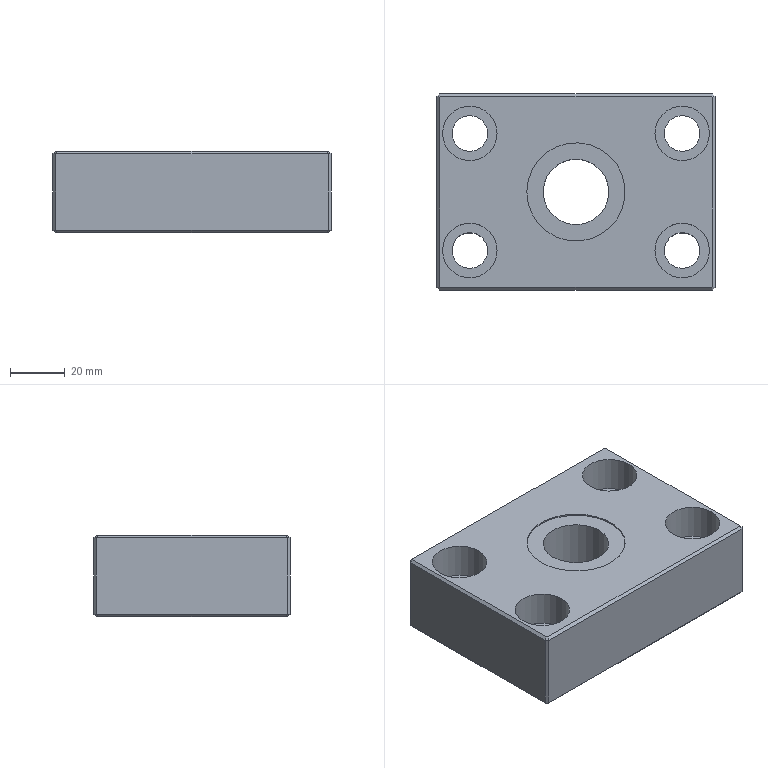NC program | NX | posted with a generic post | part box 102 x 72 x 30 mm
Whole program:
N10 G17 G21 G94 G90
(PLANAR_MILL_COPY_1 , TOOL : D80-FACE-MILL)
N12 T01 M6
N14 G54
N16 G17 G0 G90 X96. Y-0.5 S3500 M3
N18 G43 Z35. H1
N20 Z6.
N22 G94 G1 Z4. F1200.
N24 X53.
N26 X-53.
N28 X-96.
N30 Z6.
N32 G0 Z35.
N34 X96.
N36 Z5.
N38 G1 Z3.
N40 X53.
N42 X-53.
N44 X-96.
N46 Z5.
N48 G0 Z35.
N50 X96.
N52 Z4.
N54 G1 Z2.
N56 X53.
N58 X-53.
N60 X-96.
N62 Z4.
N64 G0 Z35.
N66 X96.
N68 Z3.
N70 G1 Z1.
N72 X53.
N74 X-53.
N76 X-96.
N78 Z3.
N80 G0 Z35.
N82 X96.
N84 Z2.03
N86 G1 Z0.03
N88 X53.
N90 X-53.
N92 X-96.
N94 Z2.03
N96 G0 Z35.
N98 M5
(PLANAR_MILL_5 , TOOL : D3-9-D4-50-3T-ROUGH)
N100 T09 M6
N102 G54
N104 G17 G0 G90 X-10.959 Y-26.704 S4500 M3
N106 G43 Z30. H9
N108 Z1.
N110 G94 G1 X-11.204 Y-26.618 Z0.999 F800.
N112 X-14.44 Y-25.011 Z0.99
N114 X-17.45 Y-23.012 Z0.98
N116 X-20.187 Y-20.653 Z0.971
N118 X-22.608 Y-17.97 Z0.961
N120 X-24.675 Y-15.006 Z0.952
N122 X-26.356 Y-11.807 Z0.943
N124 X-27.624 Y-8.424 Z0.933
N126 X-28.46 Y-4.908 Z0.924
N128 X-28.85 Y-1.316 Z0.914
N130 Y1.316 Z0.907
N132 X-28.46 Y4.908 Z0.898
N134 X-27.624 Y8.424 Z0.888
N136 X-26.356 Y11.807 Z0.879
N138 X-24.675 Y15.006 Z0.869
N140 X-22.608 Y17.97 Z0.86
N142 X-20.187 Y20.653 Z0.851
N144 X-17.45 Y23.012 Z0.841
N146 X-14.44 Y25.011 Z0.832
N148 X-11.204 Y26.618 Z0.822
N150 X-7.792 Y27.809 Z0.813
N152 X-4.258 Y28.564 Z0.803
N154 X-0.658 Y28.872 Z0.794
N156 X2.952 Y28.729 Z0.784
N158 X6.517 Y28.135 Z0.775
N160 X9.979 Y27.101 Z0.765
N162 X13.285 Y25.643 Z0.756
N164 X15.565 Y24.327 Z0.749
N166 X18.354 Y22.298 Z0.74
N168 X20.881 Y19.951 Z0.731
N170 X23.111 Y17.319 Z0.722
N172 X25.011 Y14.44 Z0.713
N174 X26.554 Y11.355 Z0.704
N176 X27.718 Y8.109 Z0.695
N178 X28.487 Y4.746 Z0.686
N180 X28.85 Y1.316 Z0.677
N182 Y-1.316 Z0.67
N184 X28.487 Y-4.746 Z0.661
N186 X27.718 Y-8.109 Z0.652
N188 X26.554 Y-11.355 Z0.643
N190 X25.011 Y-14.44 Z0.634
N192 X23.111 Y-17.319 Z0.625
N194 X20.881 Y-19.951 Z0.616
N196 X18.354 Y-22.298 Z0.607
N198 X15.565 Y-24.327 Z0.598
N200 X13.285 Y-25.643 Z0.591
N202 X9.979 Y-27.101 Z0.581
N204 X6.517 Y-28.135 Z0.572
N206 X2.952 Y-28.729 Z0.562
N208 X-0.658 Y-28.872 Z0.553
N210 X-4.258 Y-28.564 Z0.543
N212 X-7.792 Y-27.809 Z0.534
N214 X-11.204 Y-26.618 Z0.525
N216 X-14.44 Y-25.011 Z0.515
N218 X-17.45 Y-23.012 Z0.506
N220 X-20.187 Y-20.653 Z0.496
N222 X-22.608 Y-17.97 Z0.487
N224 X-24.675 Y-15.006 Z0.477
N226 X-26.356 Y-11.807 Z0.468
N228 X-27.624 Y-8.424 Z0.458
N230 X-28.46 Y-4.908 Z0.449
N232 X-28.85 Y-1.316 Z0.439
N234 Y1.316 Z0.433
N236 X-28.46 Y4.908 Z0.423
N238 X-27.624 Y8.424 Z0.414
N240 X-26.356 Y11.807 Z0.404
N242 X-24.675 Y15.006 Z0.395
N244 X-22.608 Y17.97 Z0.385
N246 X-20.187 Y20.653 Z0.376
N248 X-17.45 Y23.012 Z0.366
N250 X-14.44 Y25.011 Z0.357
N252 X-11.204 Y26.618 Z0.347
N254 X-7.792 Y27.809 Z0.338
N256 X-4.258 Y28.564 Z0.328
N258 X-0.658 Y28.872 Z0.319
N260 X2.952 Y28.729 Z0.31
N262 X6.517 Y28.135 Z0.3
N264 X9.979 Y27.101 Z0.291
N266 X13.285 Y25.643 Z0.281
N268 X15.565 Y24.327 Z0.274
N270 X18.354 Y22.298 Z0.265
N272 X20.881 Y19.951 Z0.256
N274 X23.111 Y17.319 Z0.247
N276 X25.011 Y14.44 Z0.238
N278 X26.554 Y11.355 Z0.229
N280 X27.718 Y8.109 Z0.22
N282 X28.487 Y4.746 Z0.211
N284 X28.85 Y1.316 Z0.202
N286 Y-1.316 Z0.195
N288 X28.487 Y-4.746 Z0.186
N290 X27.718 Y-8.109 Z0.177
N292 X26.554 Y-11.355 Z0.168
N294 X25.011 Y-14.44 Z0.159
N296 X23.111 Y-17.319 Z0.15
N298 X20.881 Y-19.951 Z0.141
N300 X18.354 Y-22.298 Z0.132
N302 X15.565 Y-24.327 Z0.123
N304 X13.285 Y-25.643 Z0.116
N306 X9.979 Y-27.101 Z0.107
N308 X6.517 Y-28.135 Z0.097
N310 X2.952 Y-28.729 Z0.088
N312 X-0.658 Y-28.872 Z0.078
N314 X-4.258 Y-28.564 Z0.069
N316 X-7.792 Y-27.809 Z0.059
N318 X-11.204 Y-26.618 Z0.05
N320 X-14.44 Y-25.011 Z0.04
N322 X-17.45 Y-23.012 Z0.031
N324 X-20.187 Y-20.653 Z0.021
N326 X-22.608 Y-17.97 Z0.012
N328 X-24.675 Y-15.006 Z0.002
N330 X-26.356 Y-11.807 Z-0.007
N332 X-27.624 Y-8.424 Z-0.016
N334 X-28.46 Y-4.908 Z-0.026
N336 X-28.85 Y-1.316 Z-0.035
N338 Y1.316 Z-0.042
N340 X-28.46 Y4.908 Z-0.052
N342 X-27.624 Y8.424 Z-0.061
N344 X-26.356 Y11.807 Z-0.071
N346 X-24.675 Y15.006 Z-0.08
N348 X-22.608 Y17.97 Z-0.09
N350 X-20.187 Y20.653 Z-0.099
N352 X-17.45 Y23.012 Z-0.108
N354 X-14.44 Y25.011 Z-0.118
N356 X-11.204 Y26.618 Z-0.127
N358 X-7.792 Y27.809 Z-0.137
N360 X-4.258 Y28.564 Z-0.146
N362 X-0.658 Y28.872 Z-0.156
N364 X2.952 Y28.729 Z-0.165
N366 X6.517 Y28.135 Z-0.175
N368 X9.979 Y27.101 Z-0.184
N370 X13.285 Y25.643 Z-0.194
N372 X15.565 Y24.327 Z-0.2
N374 X18.354 Y22.298 Z-0.21
N376 X20.881 Y19.951 Z-0.219
N378 X23.111 Y17.319 Z-0.228
N380 X25.011 Y14.44 Z-0.237
N382 X26.554 Y11.355 Z-0.246
N384 X27.718 Y8.109 Z-0.255
N386 X28.487 Y4.746 Z-0.264
N388 X28.85 Y1.316 Z-0.273
N390 Y-1.316 Z-0.28
N392 X28.487 Y-4.746 Z-0.289
N394 X27.718 Y-8.109 Z-0.298
N396 X26.554 Y-11.355 Z-0.307
N398 X25.011 Y-14.44 Z-0.316
N400 X23.111 Y-17.319 Z-0.325
N402 X20.881 Y-19.951 Z-0.334
N404 X18.354 Y-22.298 Z-0.343
N406 X15.565 Y-24.327 Z-0.352
N408 X13.285 Y-25.643 Z-0.359
N410 X9.979 Y-27.101 Z-0.368
N412 X6.517 Y-28.135 Z-0.378
N414 X2.952 Y-28.729 Z-0.387
N416 X-0.658 Y-28.872 Z-0.397
N418 X-4.258 Y-28.564 Z-0.406
N420 X-7.792 Y-27.809 Z-0.416
N422 X-11.204 Y-26.618 Z-0.425
N424 X-14.44 Y-25.011 Z-0.434
N426 X-17.45 Y-23.012 Z-0.444
N428 X-20.187 Y-20.653 Z-0.453
N430 X-22.608 Y-17.97 Z-0.463
N432 X-24.675 Y-15.006 Z-0.472
N434 X-26.356 Y-11.807 Z-0.482
N436 X-27.624 Y-8.424 Z-0.491
N438 X-28.46 Y-4.908 Z-0.501
N440 X-28.85 Y-1.316 Z-0.51
N442 Y1.316 Z-0.517
N444 X-28.46 Y4.908 Z-0.526
N446 X-27.624 Y8.424 Z-0.536
N448 X-26.356 Y11.807 Z-0.545
N450 X-24.675 Y15.006 Z-0.555
N452 X-22.608 Y17.97 Z-0.564
N454 X-20.187 Y20.653 Z-0.574
N456 X-17.45 Y23.012 Z-0.583
N458 X-14.44 Y25.011 Z-0.593
N460 X-11.204 Y26.618 Z-0.602
N462 X-7.792 Y27.809 Z-0.612
N464 X-4.258 Y28.564 Z-0.621
N466 X-0.658 Y28.872 Z-0.631
N468 X2.952 Y28.729 Z-0.64
N470 X6.517 Y28.135 Z-0.649
N472 X9.979 Y27.101 Z-0.659
N474 X13.285 Y25.643 Z-0.668
N476 X15.565 Y24.327 Z-0.675
N478 X18.354 Y22.298 Z-0.684
N480 X20.881 Y19.951 Z-0.693
N482 X23.111 Y17.319 Z-0.702
N484 X25.011 Y14.44 Z-0.711
N486 X26.554 Y11.355 Z-0.72
N488 X27.718 Y8.109 Z-0.729
N490 X28.487 Y4.746 Z-0.738
N492 X28.85 Y1.316 Z-0.747
N494 Y-1.316 Z-0.754
N496 X28.487 Y-4.746 Z-0.763
N498 X27.718 Y-8.109 Z-0.772
N500 X26.554 Y-11.355 Z-0.781
N502 X25.011 Y-14.44 Z-0.791
N504 X23.111 Y-17.319 Z-0.8
N506 X20.881 Y-19.951 Z-0.809
N508 X18.354 Y-22.298 Z-0.818
N510 X15.565 Y-24.327 Z-0.827
N512 X13.285 Y-25.643 Z-0.834
N514 X9.979 Y-27.101 Z-0.843
N516 X6.517 Y-28.135 Z-0.852
N518 X2.952 Y-28.729 Z-0.862
N520 X-0.658 Y-28.872 Z-0.871
N522 X-4.258 Y-28.564 Z-0.881
N524 X-7.792 Y-27.809 Z-0.89
N526 X-11.204 Y-26.618 Z-0.9
N528 X-14.44 Y-25.011 Z-0.909
N530 X-17.45 Y-23.012 Z-0.919
N532 X-20.187 Y-20.653 Z-0.928
N534 X-22.608 Y-17.97 Z-0.938
N536 X-24.675 Y-15.006 Z-0.947
N538 X-26.356 Y-11.807 Z-0.956
N540 X-27.624 Y-8.424 Z-0.966
N542 X-28.46 Y-4.908 Z-0.975
N544 X-28.85 Y-1.316 Z-0.985
N546 Y1.316 Z-0.992
N548 X-28.46 Y4.908 Z-1.001
N550 X-27.624 Y8.424 Z-1.011
N552 X-26.356 Y11.807 Z-1.02
N554 X-24.675 Y15.006 Z-1.03
N556 X-22.608 Y17.97 Z-1.039
N558 X-20.187 Y20.653 Z-1.049
N560 X-17.45 Y23.012 Z-1.058
N562 X-14.44 Y25.011 Z-1.067
N564 X-11.204 Y26.618 Z-1.077
N566 X-7.792 Y27.809 Z-1.086
N568 X-4.258 Y28.564 Z-1.096
N570 X-0.658 Y28.872 Z-1.105
N572 X2.952 Y28.729 Z-1.115
N574 X6.517 Y28.135 Z-1.124
N576 X9.979 Y27.101 Z-1.134
N578 X13.285 Y25.643 Z-1.143
N580 X15.565 Y24.327 Z-1.15
N582 X18.354 Y22.298 Z-1.159
N584 X20.881 Y19.951 Z-1.168
N586 X23.111 Y17.319 Z-1.177
N588 X25.011 Y14.44 Z-1.186
N590 X26.554 Y11.355 Z-1.195
N592 X27.718 Y8.109 Z-1.204
N594 X28.487 Y4.746 Z-1.213
N596 X28.85 Y1.316 Z-1.222
N598 Y-1.316 Z-1.229
N600 X28.487 Y-4.746 Z-1.238
N602 X27.718 Y-8.109 Z-1.247
N604 X26.554 Y-11.355 Z-1.256
N606 X25.011 Y-14.44 Z-1.265
N608 X23.111 Y-17.319 Z-1.274
N610 X20.881 Y-19.951 Z-1.283
N612 X18.354 Y-22.298 Z-1.292
N614 X15.565 Y-24.327 Z-1.301
N616 X13.285 Y-25.643 Z-1.308
N618 X9.979 Y-27.101 Z-1.318
N620 X6.517 Y-28.135 Z-1.327
N622 X2.952 Y-28.729 Z-1.337
N624 X-0.658 Y-28.872 Z-1.346
N626 X-4.258 Y-28.564 Z-1.356
N628 X-7.792 Y-27.809 Z-1.365
N630 X-11.204 Y-26.618 Z-1.375
N632 X-14.44 Y-25.011 Z-1.384
N634 X-17.45 Y-23.012 Z-1.393
N636 X-20.187 Y-20.653 Z-1.403
N638 X-22.608 Y-17.97 Z-1.412
N640 X-24.675 Y-15.006 Z-1.422
N642 X-26.356 Y-11.807 Z-1.431
N644 X-27.624 Y-8.424 Z-1.441
N646 X-28.46 Y-4.908 Z-1.45
N648 X-28.85 Y-1.316 Z-1.46
N650 Y1.316 Z-1.467
N652 X-28.46 Y4.908 Z-1.476
N654 X-27.624 Y8.424 Z-1.485
N656 X-26.356 Y11.807 Z-1.495
N658 X-24.675 Y15.006 Z-1.504
N660 X-22.608 Y17.97 Z-1.514
N662 X-20.187 Y20.653 Z-1.523
N664 X-17.45 Y23.012 Z-1.533
N666 X-14.44 Y25.011 Z-1.542
N668 X-11.204 Y26.618 Z-1.552
N670 X-7.792 Y27.809 Z-1.561
N672 X-4.258 Y28.564 Z-1.571
N674 X-0.658 Y28.872 Z-1.58
N676 X2.952 Y28.729 Z-1.59
N678 X6.517 Y28.135 Z-1.599
N680 X9.979 Y27.101 Z-1.608
N682 X13.285 Y25.643 Z-1.618
N684 X15.565 Y24.327 Z-1.625
N686 X18.354 Y22.298 Z-1.634
N688 X20.881 Y19.951 Z-1.643
N690 X23.111 Y17.319 Z-1.652
N692 X25.011 Y14.44 Z-1.661
N694 X26.554 Y11.355 Z-1.67
N696 X27.718 Y8.109 Z-1.679
N698 X28.487 Y4.746 Z-1.688
N700 X28.85 Y1.316 Z-1.697
N702 Y-1.316 Z-1.704
N704 X28.487 Y-4.746 Z-1.713
N706 X27.718 Y-8.109 Z-1.722
N708 X26.554 Y-11.355 Z-1.731
N710 X25.011 Y-14.44 Z-1.74
N712 X23.111 Y-17.319 Z-1.749
N714 X20.881 Y-19.951 Z-1.758
N716 X18.354 Y-22.298 Z-1.767
N718 X15.565 Y-24.327 Z-1.776
N720 X13.285 Y-25.643 Z-1.783
N722 X9.979 Y-27.101 Z-1.793
N724 X6.517 Y-28.135 Z-1.802
N726 X2.952 Y-28.729 Z-1.811
N728 X-0.658 Y-28.872 Z-1.821
N730 X-4.258 Y-28.564 Z-1.83
N732 X-7.792 Y-27.809 Z-1.84
N734 X-11.204 Y-26.618 Z-1.849
N736 X-14.44 Y-25.011 Z-1.859
N738 X-17.45 Y-23.012 Z-1.868
N740 X-20.187 Y-20.653 Z-1.878
N742 X-22.608 Y-17.97 Z-1.887
N744 X-24.675 Y-15.006 Z-1.897
N746 X-26.356 Y-11.807 Z-1.906
N748 X-27.624 Y-8.424 Z-1.915
N750 X-28.46 Y-4.908 Z-1.925
N752 X-28.85 Y-1.316 Z-1.934
N754 Y1.316 Z-1.941
N756 X-28.46 Y4.908 Z-1.951
N758 X-27.624 Y8.424 Z-1.96
N760 X-26.356 Y11.807 Z-1.97
N762 X-24.675 Y15.006 Z-1.979
N764 X-22.608 Y17.97 Z-1.989
N766 X-20.187 Y20.653 Z-1.998
N768 X-17.45 Y23.012 Z-2.008
N770 X-14.44 Y25.011 Z-2.017
N772 X-11.204 Y26.618 Z-2.026
N774 X-7.792 Y27.809 Z-2.036
N776 X-4.258 Y28.564 Z-2.045
N778 X-0.658 Y28.872 Z-2.055
N780 X2.952 Y28.729 Z-2.064
N782 X6.517 Y28.135 Z-2.074
N784 X9.979 Y27.101 Z-2.083
N786 X13.285 Y25.643 Z-2.093
N788 X15.565 Y24.327 Z-2.1
N790 X18.354 Y22.298 Z-2.109
N792 X20.881 Y19.951 Z-2.118
N794 X23.111 Y17.319 Z-2.127
N796 X25.011 Y14.44 Z-2.136
N798 X26.554 Y11.355 Z-2.145
N800 X27.718 Y8.109 Z-2.154
N802 X28.487 Y4.746 Z-2.163
N804 X28.85 Y1.316 Z-2.172
N806 Y-1.316 Z-2.179
N808 X28.487 Y-4.746 Z-2.188
N810 X27.718 Y-8.109 Z-2.197
N812 X26.554 Y-11.355 Z-2.206
N814 X25.011 Y-14.44 Z-2.215
N816 X23.111 Y-17.319 Z-2.224
N818 X20.881 Y-19.951 Z-2.233
N820 X18.354 Y-22.298 Z-2.242
N822 X15.565 Y-24.327 Z-2.251
N824 X13.285 Y-25.643 Z-2.258
N826 X9.979 Y-27.101 Z-2.267
N828 X6.517 Y-28.135 Z-2.277
N830 X2.952 Y-28.729 Z-2.286
N832 X-0.658 Y-28.872 Z-2.296
N834 X-4.258 Y-28.564 Z-2.305
N836 X-7.792 Y-27.809 Z-2.315
N838 X-11.204 Y-26.618 Z-2.324
N840 X-14.44 Y-25.011 Z-2.333
N842 X-17.45 Y-23.012 Z-2.343
N844 X-20.187 Y-20.653 Z-2.352
N846 X-22.608 Y-17.97 Z-2.362
N848 X-24.675 Y-15.006 Z-2.371
N850 X-26.356 Y-11.807 Z-2.381
N852 X-27.624 Y-8.424 Z-2.39
N854 X-28.46 Y-4.908 Z-2.4
N856 X-28.85 Y-1.316 Z-2.409
N858 Y1.316 Z-2.416
N860 X-28.46 Y4.908 Z-2.426
N862 X-27.624 Y8.424 Z-2.435
N864 X-26.356 Y11.807 Z-2.444
N866 X-24.675 Y15.006 Z-2.454
N868 X-22.608 Y17.97 Z-2.463
N870 X-20.187 Y20.653 Z-2.473
N872 X-17.45 Y23.012 Z-2.482
N874 X-14.44 Y25.011 Z-2.492
N876 X-11.204 Y26.618 Z-2.501
N878 X-7.792 Y27.809 Z-2.511
N880 X-4.258 Y28.564 Z-2.52
N882 X-0.658 Y28.872 Z-2.53
N884 X2.952 Y28.729 Z-2.539
N886 X6.517 Y28.135 Z-2.549
N888 X9.979 Y27.101 Z-2.558
N890 X13.285 Y25.643 Z-2.567
N892 X15.565 Y24.327 Z-2.574
N894 X18.354 Y22.298 Z-2.583
N896 X20.881 Y19.951 Z-2.592
N898 X23.111 Y17.319 Z-2.601
N900 X25.011 Y14.44 Z-2.61
N902 X26.554 Y11.355 Z-2.619
N904 X27.718 Y8.109 Z-2.628
N906 X28.487 Y4.746 Z-2.638
N908 X28.85 Y1.316 Z-2.647
N910 Y0. Z-2.65
N912 G2 X0. Y-28.85 R28.85
N914 X28.85 Y0. R-28.85
N916 G1 Z-1.65
N918 G0 Z30.
(PLANAR_MILL_5_COPY , TOOL : D3-9-D4-50-3T-ROUGH)
N920 X-18.753 Y-23.602
N922 Z1.
N924 G1 X-18.239 Y-24.045 Z0.998
N926 X-15.09 Y-26.137 Z0.988
N928 X-11.705 Y-27.818 Z0.978
N930 X-8.136 Y-29.063 Z0.969
N932 X-4.439 Y-29.852 Z0.959
N934 X-0.673 Y-30.173 Z0.949
N936 X3.104 Y-30.02 Z0.939
N938 X6.832 Y-29.397 Z0.929
N940 X10.453 Y-28.312 Z0.919
N942 X13.91 Y-26.783 Z0.909
N944 X16.24 Y-25.438 Z0.902
N946 X19.163 Y-23.316 Z0.893
N948 X21.811 Y-20.859 Z0.883
N950 X24.147 Y-18.104 Z0.874
N952 X26.137 Y-15.09 Z0.864
N954 X27.752 Y-11.859 Z0.855
N956 X28.97 Y-8.459 Z0.845
N958 X29.773 Y-4.938 Z0.836
N960 X30.15 Y-1.345 Z0.826
N962 Y1.345 Z0.819
N964 X29.773 Y4.938 Z0.81
N966 X28.97 Y8.459 Z0.801
N968 X27.752 Y11.859 Z0.791
N970 X26.137 Y15.09 Z0.782
N972 X24.147 Y18.104 Z0.772
N974 X21.811 Y20.859 Z0.763
N976 X19.163 Y23.316 Z0.753
N978 X16.24 Y25.438 Z0.744
N980 X13.91 Y26.783 Z0.737
N982 X10.453 Y28.312 Z0.727
N984 X6.832 Y29.397 Z0.717
N986 X3.104 Y30.02 Z0.707
N988 X-0.673 Y30.173 Z0.697
N990 X-4.439 Y29.852 Z0.687
N992 X-8.136 Y29.063 Z0.677
N994 X-11.705 Y27.818 Z0.667
N996 X-15.09 Y26.137 Z0.658
N998 X-18.239 Y24.045 Z0.648
N1000 X-21.101 Y21.577 Z0.638
N1002 X-23.633 Y18.77 Z0.628
N1004 X-25.794 Y15.669 Z0.618
N1006 X-27.55 Y12.322 Z0.608
N1008 X-28.874 Y8.782 Z0.598
N1010 X-29.745 Y5.103 Z0.588
N1012 X-30.15 Y1.345 Z0.578
N1014 Y-1.345 Z0.571
N1016 X-29.745 Y-5.103 Z0.561
N1018 X-28.874 Y-8.782 Z0.552
N1020 X-27.55 Y-12.322 Z0.542
N1022 X-25.794 Y-15.669 Z0.532
N1024 X-23.633 Y-18.77 Z0.522
N1026 X-21.101 Y-21.577 Z0.512
N1028 X-18.239 Y-24.045 Z0.502
N1030 X-15.09 Y-26.137 Z0.492
N1032 X-11.705 Y-27.818 Z0.482
N1034 X-8.136 Y-29.063 Z0.472
N1036 X-4.439 Y-29.852 Z0.463
N1038 X-0.673 Y-30.173 Z0.453
N1040 X3.104 Y-30.02 Z0.443
N1042 X6.832 Y-29.397 Z0.433
N1044 X10.453 Y-28.312 Z0.423
N1046 X13.91 Y-26.783 Z0.413
N1048 X16.24 Y-25.438 Z0.406
N1050 X19.163 Y-23.316 Z0.397
N1052 X21.811 Y-20.859 Z0.387
N1054 X24.147 Y-18.104 Z0.378
N1056 X26.137 Y-15.09 Z0.368
N1058 X27.752 Y-11.859 Z0.359
N1060 X28.97 Y-8.459 Z0.349
N1062 X29.773 Y-4.938 Z0.34
N1064 X30.15 Y-1.345 Z0.33
N1066 Y1.345 Z0.323
N1068 X29.773 Y4.938 Z0.314
N1070 X28.97 Y8.459 Z0.304
N1072 X27.752 Y11.859 Z0.295
N1074 X26.137 Y15.09 Z0.285
N1076 X24.147 Y18.104 Z0.276
N1078 X21.811 Y20.859 Z0.267
N1080 X19.163 Y23.316 Z0.257
N1082 X16.24 Y25.438 Z0.248
N1084 X13.91 Y26.783 Z0.241
N1086 X10.453 Y28.312 Z0.231
N1088 X6.832 Y29.397 Z0.221
N1090 X3.104 Y30.02 Z0.211
N1092 X-0.673 Y30.173 Z0.201
N1094 X-4.439 Y29.852 Z0.191
N1096 X-8.136 Y29.063 Z0.181
N1098 X-11.705 Y27.818 Z0.171
N1100 X-15.09 Y26.137 Z0.161
N1102 X-18.239 Y24.045 Z0.152
N1104 X-21.101 Y21.577 Z0.142
N1106 X-23.633 Y18.77 Z0.132
N1108 X-25.794 Y15.669 Z0.122
N1110 X-27.55 Y12.322 Z0.112
N1112 X-28.874 Y8.782 Z0.102
N1114 X-29.745 Y5.103 Z0.092
N1116 X-30.15 Y1.345 Z0.082
N1118 Y-1.345 Z0.075
N1120 X-29.745 Y-5.103 Z0.065
N1122 X-28.874 Y-8.782 Z0.055
N1124 X-27.55 Y-12.322 Z0.046
N1126 X-25.794 Y-15.669 Z0.036
N1128 X-23.633 Y-18.77 Z0.026
N1130 X-21.101 Y-21.577 Z0.016
N1132 X-18.239 Y-24.045 Z0.006
N1134 X-15.09 Y-26.137 Z-0.004
N1136 X-11.705 Y-27.818 Z-0.014
N1138 X-8.136 Y-29.063 Z-0.024
N1140 X-4.439 Y-29.852 Z-0.034
N1142 X-0.673 Y-30.173 Z-0.044
N1144 X3.104 Y-30.02 Z-0.053
N1146 X6.832 Y-29.397 Z-0.063
N1148 X10.453 Y-28.312 Z-0.073
N1150 X13.91 Y-26.783 Z-0.083
N1152 X16.24 Y-25.438 Z-0.09
N1154 X19.163 Y-23.316 Z-0.1
N1156 X21.811 Y-20.859 Z-0.109
N1158 X24.147 Y-18.104 Z-0.119
N1160 X26.137 Y-15.09 Z-0.128
N1162 X27.752 Y-11.859 Z-0.137
N1164 X28.97 Y-8.459 Z-0.147
N1166 X29.773 Y-4.938 Z-0.156
N1168 X30.15 Y-1.345 Z-0.166
N1170 Y1.345 Z-0.173
N1172 X29.773 Y4.938 Z-0.182
N1174 X28.97 Y8.459 Z-0.192
N1176 X27.752 Y11.859 Z-0.201
N1178 X26.137 Y15.09 Z-0.211
N1180 X24.147 Y18.104 Z-0.22
N1182 X21.811 Y20.859 Z-0.23
N1184 X19.163 Y23.316 Z-0.239
N1186 X16.24 Y25.438 Z-0.248
N1188 X13.91 Y26.783 Z-0.256
N1190 X10.453 Y28.312 Z-0.265
N1192 X6.832 Y29.397 Z-0.275
N1194 X3.104 Y30.02 Z-0.285
N1196 X-0.673 Y30.173 Z-0.295
N1198 X-4.439 Y29.852 Z-0.305
N1200 X-8.136 Y29.063 Z-0.315
N1202 X-11.705 Y27.818 Z-0.325
N1204 X-15.09 Y26.137 Z-0.335
N1206 X-18.239 Y24.045 Z-0.345
N1208 X-21.101 Y21.577 Z-0.354
N1210 X-23.633 Y18.77 Z-0.364
N1212 X-25.794 Y15.669 Z-0.374
N1214 X-27.55 Y12.322 Z-0.384
N1216 X-28.874 Y8.782 Z-0.394
N1218 X-29.745 Y5.103 Z-0.404
N1220 X-30.15 Y1.345 Z-0.414
N1222 Y-1.345 Z-0.421
N1224 X-29.745 Y-5.103 Z-0.431
N1226 X-28.874 Y-8.782 Z-0.441
N1228 X-27.55 Y-12.322 Z-0.451
N1230 X-25.794 Y-15.669 Z-0.46
N1232 X-23.633 Y-18.77 Z-0.47
N1234 X-21.101 Y-21.577 Z-0.48
N1236 X-18.239 Y-24.045 Z-0.49
N1238 X-15.09 Y-26.137 Z-0.5
N1240 X-11.705 Y-27.818 Z-0.51
N1242 X-8.136 Y-29.063 Z-0.52
N1244 X-4.439 Y-29.852 Z-0.53
N1246 X-0.673 Y-30.173 Z-0.54
N1248 X3.104 Y-30.02 Z-0.55
N1250 X6.832 Y-29.397 Z-0.559
N1252 X10.453 Y-28.312 Z-0.569
N1254 X13.91 Y-26.783 Z-0.579
N1256 X16.24 Y-25.438 Z-0.586
N1258 X19.163 Y-23.316 Z-0.596
N1260 X21.811 Y-20.859 Z-0.605
N1262 X24.147 Y-18.104 Z-0.615
N1264 X26.137 Y-15.09 Z-0.624
N1266 X27.752 Y-11.859 Z-0.634
N1268 X28.97 Y-8.459 Z-0.643
N1270 X29.773 Y-4.938 Z-0.652
N1272 X30.15 Y-1.345 Z-0.662
N1274 Y1.345 Z-0.669
N1276 X29.773 Y4.938 Z-0.678
N1278 X28.97 Y8.459 Z-0.688
N1280 X27.752 Y11.859 Z-0.697
N1282 X26.137 Y15.09 Z-0.707
N1284 X24.147 Y18.104 Z-0.716
N1286 X21.811 Y20.859 Z-0.726
N1288 X19.163 Y23.316 Z-0.735
N1290 X16.24 Y25.438 Z-0.745
N1292 X13.91 Y26.783 Z-0.752
N1294 X10.453 Y28.312 Z-0.762
N1296 X6.832 Y29.397 Z-0.771
N1298 X3.104 Y30.02 Z-0.781
N1300 X-0.673 Y30.173 Z-0.791
N1302 X-4.439 Y29.852 Z-0.801
N1304 X-8.136 Y29.063 Z-0.811
N1306 X-11.705 Y27.818 Z-0.821
N1308 X-15.09 Y26.137 Z-0.831
N1310 X-18.239 Y24.045 Z-0.841
N1312 X-21.101 Y21.577 Z-0.851
N1314 X-23.633 Y18.77 Z-0.861
N1316 X-25.794 Y15.669 Z-0.87
N1318 X-27.55 Y12.322 Z-0.88
N1320 X-28.874 Y8.782 Z-0.89
N1322 X-29.745 Y5.103 Z-0.9
N1324 X-30.15 Y1.345 Z-0.91
N1326 Y-1.345 Z-0.917
N1328 X-29.745 Y-5.103 Z-0.927
N1330 X-28.874 Y-8.782 Z-0.937
N1332 X-27.55 Y-12.322 Z-0.947
N1334 X-25.794 Y-15.669 Z-0.957
N1336 X-23.633 Y-18.77 Z-0.967
N1338 X-21.101 Y-21.577 Z-0.976
N1340 X-18.239 Y-24.045 Z-0.986
N1342 X-15.09 Y-26.137 Z-0.996
N1344 X-11.705 Y-27.818 Z-1.006
N1346 X-8.136 Y-29.063 Z-1.016
N1348 X-4.439 Y-29.852 Z-1.026
N1350 X-0.673 Y-30.173 Z-1.036
N1352 X3.104 Y-30.02 Z-1.046
N1354 X6.832 Y-29.397 Z-1.056
N1356 X10.453 Y-28.312 Z-1.065
N1358 X13.91 Y-26.783 Z-1.075
N1360 X16.24 Y-25.438 Z-1.082
N1362 X19.163 Y-23.316 Z-1.092
N1364 X21.811 Y-20.859 Z-1.101
N1366 X24.147 Y-18.104 Z-1.111
N1368 X26.137 Y-15.09 Z-1.12
N1370 X27.752 Y-11.859 Z-1.13
N1372 X28.97 Y-8.459 Z-1.139
N1374 X29.773 Y-4.938 Z-1.149
N1376 X30.15 Y-1.345 Z-1.158
N1378 Y1.345 Z-1.165
N1380 X29.773 Y4.938 Z-1.175
N1382 X28.97 Y8.459 Z-1.184
N1384 X27.752 Y11.859 Z-1.193
N1386 X26.137 Y15.09 Z-1.203
N1388 X24.147 Y18.104 Z-1.212
N1390 X21.811 Y20.859 Z-1.222
N1392 X19.163 Y23.316 Z-1.231
N1394 X16.24 Y25.438 Z-1.241
N1396 X13.91 Y26.783 Z-1.248
N1398 X10.453 Y28.312 Z-1.258
N1400 X6.832 Y29.397 Z-1.268
N1402 X3.104 Y30.02 Z-1.277
N1404 X-0.673 Y30.173 Z-1.287
N1406 X-4.439 Y29.852 Z-1.297
N1408 X-8.136 Y29.063 Z-1.307
N1410 X-11.705 Y27.818 Z-1.317
N1412 X-15.09 Y26.137 Z-1.327
N1414 X-18.239 Y24.045 Z-1.337
N1416 X-21.101 Y21.577 Z-1.347
N1418 X-23.633 Y18.77 Z-1.357
N1420 X-25.794 Y15.669 Z-1.367
N1422 X-27.55 Y12.322 Z-1.376
N1424 X-28.874 Y8.782 Z-1.386
N1426 X-29.745 Y5.103 Z-1.396
N1428 X-30.15 Y1.345 Z-1.406
N1430 Y-1.345 Z-1.413
N1432 X-29.745 Y-5.103 Z-1.423
N1434 X-28.874 Y-8.782 Z-1.433
N1436 X-27.55 Y-12.322 Z-1.443
N1438 X-25.794 Y-15.669 Z-1.453
N1440 X-23.633 Y-18.77 Z-1.463
N1442 X-21.101 Y-21.577 Z-1.473
N1444 X-18.239 Y-24.045 Z-1.482
N1446 X-15.09 Y-26.137 Z-1.492
N1448 X-11.705 Y-27.818 Z-1.502
N1450 X-8.136 Y-29.063 Z-1.512
N1452 X-4.439 Y-29.852 Z-1.522
N1454 X-0.673 Y-30.173 Z-1.532
N1456 X3.104 Y-30.02 Z-1.542
N1458 X6.832 Y-29.397 Z-1.552
N1460 X10.453 Y-28.312 Z-1.562
N1462 X13.91 Y-26.783 Z-1.572
N1464 X16.24 Y-25.438 Z-1.579
N1466 X19.163 Y-23.316 Z-1.588
N1468 X21.811 Y-20.859 Z-1.597
N1470 X24.147 Y-18.104 Z-1.607
N1472 X26.137 Y-15.09 Z-1.616
N1474 X27.752 Y-11.859 Z-1.626
N1476 X28.97 Y-8.459 Z-1.635
N1478 X29.773 Y-4.938 Z-1.645
N1480 X30.15 Y-1.345 Z-1.654
N1482 Y1.345 Z-1.661
N1484 X29.773 Y4.938 Z-1.671
N1486 X28.97 Y8.459 Z-1.68
N1488 X27.752 Y11.859 Z-1.69
N1490 X26.137 Y15.09 Z-1.699
N1492 X24.147 Y18.104 Z-1.709
N1494 X21.811 Y20.859 Z-1.718
N1496 X19.163 Y23.316 Z-1.727
N1498 X16.24 Y25.438 Z-1.737
N1500 X13.91 Y26.783 Z-1.744
N1502 X10.453 Y28.312 Z-1.754
N1504 X6.832 Y29.397 Z-1.764
N1506 X3.104 Y30.02 Z-1.774
N1508 X-0.673 Y30.173 Z-1.784
N1510 X-4.439 Y29.852 Z-1.793
N1512 X-8.136 Y29.063 Z-1.803
N1514 X-11.705 Y27.818 Z-1.813
N1516 X-15.09 Y26.137 Z-1.823
N1518 X-18.239 Y24.045 Z-1.833
N1520 X-21.101 Y21.577 Z-1.843
N1522 X-23.633 Y18.77 Z-1.853
N1524 X-25.794 Y15.669 Z-1.863
N1526 X-27.55 Y12.322 Z-1.873
N1528 X-28.874 Y8.782 Z-1.882
N1530 X-29.745 Y5.103 Z-1.892
N1532 X-30.15 Y1.345 Z-1.902
N1534 Y-1.345 Z-1.909
N1536 X-29.745 Y-5.103 Z-1.919
N1538 X-28.874 Y-8.782 Z-1.929
N1540 X-27.55 Y-12.322 Z-1.939
N1542 X-25.794 Y-15.669 Z-1.949
N1544 X-23.633 Y-18.77 Z-1.959
N1546 X-21.101 Y-21.577 Z-1.969
N1548 X-18.239 Y-24.045 Z-1.979
N1550 X-15.09 Y-26.137 Z-1.988
N1552 X-11.705 Y-27.818 Z-1.998
N1554 X-8.136 Y-29.063 Z-2.008
N1556 X-4.439 Y-29.852 Z-2.018
N1558 X-0.673 Y-30.173 Z-2.028
N1560 X3.104 Y-30.02 Z-2.038
N1562 X6.832 Y-29.397 Z-2.048
N1564 X10.453 Y-28.312 Z-2.058
N1566 X13.91 Y-26.783 Z-2.068
N1568 X16.24 Y-25.438 Z-2.075
N1570 X19.163 Y-23.316 Z-2.084
N1572 X21.811 Y-20.859 Z-2.094
N1574 X24.147 Y-18.104 Z-2.103
N1576 X26.137 Y-15.09 Z-2.113
N1578 X27.752 Y-11.859 Z-2.122
N1580 X28.97 Y-8.459 Z-2.131
N1582 X29.773 Y-4.938 Z-2.141
N1584 X30.15 Y-1.345 Z-2.15
N1586 Y1.345 Z-2.157
N1588 X29.773 Y4.938 Z-2.167
N1590 X28.97 Y8.459 Z-2.176
N1592 X27.752 Y11.859 Z-2.186
N1594 X26.137 Y15.09 Z-2.195
N1596 X24.147 Y18.104 Z-2.205
N1598 X21.811 Y20.859 Z-2.214
N1600 X19.163 Y23.316 Z-2.224
N1602 X16.24 Y25.438 Z-2.233
N1604 X13.91 Y26.783 Z-2.24
N1606 X10.453 Y28.312 Z-2.25
N1608 X6.832 Y29.397 Z-2.26
N1610 X3.104 Y30.02 Z-2.27
N1612 X-0.673 Y30.173 Z-2.28
N1614 X-4.439 Y29.852 Z-2.29
N1616 X-8.136 Y29.063 Z-2.299
N1618 X-11.705 Y27.818 Z-2.309
N1620 X-15.09 Y26.137 Z-2.319
N1622 X-18.239 Y24.045 Z-2.329
N1624 X-21.101 Y21.577 Z-2.339
N1626 X-23.633 Y18.77 Z-2.349
N1628 X-25.794 Y15.669 Z-2.359
N1630 X-27.55 Y12.322 Z-2.369
N1632 X-28.874 Y8.782 Z-2.379
N1634 X-29.745 Y5.103 Z-2.389
N1636 X-30.15 Y1.345 Z-2.398
N1638 Y-1.345 Z-2.405
N1640 X-29.745 Y-5.103 Z-2.415
N1642 X-28.874 Y-8.782 Z-2.425
N1644 X-27.55 Y-12.322 Z-2.435
N1646 X-25.794 Y-15.669 Z-2.445
N1648 X-23.633 Y-18.77 Z-2.455
N1650 X-21.101 Y-21.577 Z-2.465
N1652 X-18.239 Y-24.045 Z-2.475
N1654 X-15.09 Y-26.137 Z-2.485
N1656 X-11.705 Y-27.818 Z-2.495
N1658 X-8.136 Y-29.063 Z-2.504
N1660 X-4.439 Y-29.852 Z-2.514
N1662 X-0.673 Y-30.173 Z-2.524
N1664 X3.104 Y-30.02 Z-2.534
N1666 X6.832 Y-29.397 Z-2.544
N1668 X10.453 Y-28.312 Z-2.554
N1670 X13.91 Y-26.783 Z-2.564
N1672 X16.24 Y-25.438 Z-2.571
N1674 X19.163 Y-23.316 Z-2.58
N1676 X21.811 Y-20.859 Z-2.59
N1678 X24.147 Y-18.104 Z-2.599
N1680 X26.137 Y-15.09 Z-2.609
N1682 X27.752 Y-11.859 Z-2.618
N1684 X28.97 Y-8.459 Z-2.628
N1686 X29.773 Y-4.938 Z-2.637
N1688 X30.15 Y-1.345 Z-2.646
N1690 Y0. Z-2.65
N1692 G3 X0. Y30.15 R30.15
N1694 X30.15 Y0. R-30.15
N1696 G1 Z-1.65
N1698 G0 Z30.
N1700 M5
(PLANAR_MILL_5_COPY_1 , TOOL : D3-9-D4-50-3T-FINISH)
N1702 T10 M6
N1704 G54
N1706 G17 G0 G90 X29.75 Y1. S4000 M3
N1708 G43 Z30. H10
N1710 Z-0.75
N1712 G94 G1 Z-2.75 F800.
N1714 G3 X28.75 Y0. R1.
N1716 G2 X0. Y-28.75 R28.75
N1718 X28.75 Y0. R-28.75
N1720 G3 X29.75 Y-1. R1.
N1722 G1 Z-0.75
N1724 G0 Z30.
(PLANAR_MILL_5_COPY_COPY , TOOL : D3-9-D4-50-3T-FINISH)
N1726 X29.233
N1728 Z-0.75
N1730 G1 Z-2.75
N1732 X29.25
N1734 G3 X30.25 Y0. R1.
N1736 X0. Y30.25 R30.25
N1738 X30.25 Y0. R-30.25
N1740 X29.233 Y1. R1.
N1742 G1 Z-0.75
N1744 G0 Z30.
N1746 M5
(PLANAR_MILL_6 , TOOL : CHAMFER-D6-90DEG)
N1748 T05 M6
N1750 G54
N1752 G17 G0 G90 X34.4 Y-21.45 S3500 M3
N1754 G43 Z30. H5
N1756 Z1.
N1758 G94 G1 Z-1. F1000.
N1760 X33.4
N1762 G3 X38.9 Y-26.95 R5.5
N1764 X33.4 Y-21.45 R-5.5
N1766 G1 X34.4
N1768 Z1.
N1770 G0 Z30.
N1772 Y21.45
N1774 Z1.
N1776 G1 Z-1.
N1778 X33.4
N1780 G3 X38.9 Y15.95 R5.5
N1782 X33.4 Y21.45 R-5.5
N1784 G1 X34.4
N1786 Z1.
N1788 G0 Z30.
N1790 X-9.99 Y0.454
N1792 Z1.
N1794 G1 Z-1.
N1796 X-11. Y0.5
N1798 Y0.
N1800 G3 X0. Y-11. R11.
N1802 X-11. Y0. R-11.
N1804 G1 Y-0.5
N1806 X-9.99 Y-0.454
N1808 Z1.
N1810 G0 Z30.
N1812 X-43.4 Y21.45
N1814 Z1.
N1816 G1 Z-1.
N1818 X-44.4
N1820 G3 X-38.9 Y15.95 R5.5
N1822 X-44.4 Y21.45 R-5.5
N1824 G1 X-43.4
N1826 Z1.
N1828 G0 Z30.
N1830 Y-21.45
N1832 Z1.
N1834 G1 Z-1.
N1836 X-44.4
N1838 G3 X-38.9 Y-26.95 R5.5
N1840 X-44.4 Y-21.45 R-5.5
N1842 G1 X-43.4
N1844 Z1.
N1846 G0 Z30.
(PLANAR_MILL_6_COPY , TOOL : CHAMFER-D6-90DEG)
N1848 X29.746 Y-0.484
N1850 Z1.
N1852 G1 Z-1.
N1854 X30.75 Y-0.5
N1856 Y0.
N1858 G3 X0. Y30.75 R30.75
N1860 X30.75 Y0. R-30.75
N1862 G1 Y0.5
N1864 X29.746 Y0.484
N1866 Z1.
N1868 G0 Z30.
(PLANAR_MILL_6_COPY_COPY , TOOL : CHAMFER-D6-90DEG)
N1870 X29.232 Y1.035
N1872 Z1.
N1874 G1 Z-1.
N1876 X28.25 Y1.
N1878 Y0.
N1880 G2 X0. Y-28.25 R28.25
N1882 X28.25 Y0. R-28.25
N1884 G1 Y-1.
N1886 X29.232 Y-1.035
N1888 Z1.
N1890 G0 Z30.
(PLANAR_MILL_6_COPY_COPY_COPY , TOOL : CHAMFER-D6-90DEG)
N1892 X1. Y-38.5
N1894 Z-0.3
N1896 G1 Z-2.3
N1898 Y-37.5
N1900 X0.
N1902 X-49.669
N1904 G2 X-51.295 Y-36.826 R2.3
N1906 G1 X-51.826 Y-36.295
N1908 G2 X-52.5 Y-34.669 R2.3
N1910 G1 Y34.669
N1912 G2 X-51.826 Y36.295 R2.3
N1914 G1 X-51.295 Y36.826
N1916 G2 X-49.669 Y37.5 R2.3
N1918 G1 X49.669
N1920 G2 X51.295 Y36.826 R2.3
N1922 G1 X51.826 Y36.295
N1924 G2 X52.5 Y34.669 R2.3
N1926 G1 Y-34.669
N1928 G2 X51.826 Y-36.295 R2.3
N1930 G1 X51.295 Y-36.826
N1932 G2 X49.669 Y-37.5 R2.3
N1934 G1 X0.
N1936 X-1.
N1938 Y-38.5
N1940 Z-0.3
N1942 G0 Z30.
N1944 M5
(PLANAR_MILL_COPY_1_COPY , TOOL : D80-FACE-MILL)
N1946 T01 M6
N1948 G54
N1950 G17 G0 G90 X96. Y-0.5 S3500 M3
N1952 G43 Z35. H1
N1954 Z2.
N1956 G94 G1 Z0. F800.
N1958 X53.
N1960 X-53.
N1962 X-96.
N1964 Z2.
N1966 G0 Z35.
N1968 M5
N1970 M2